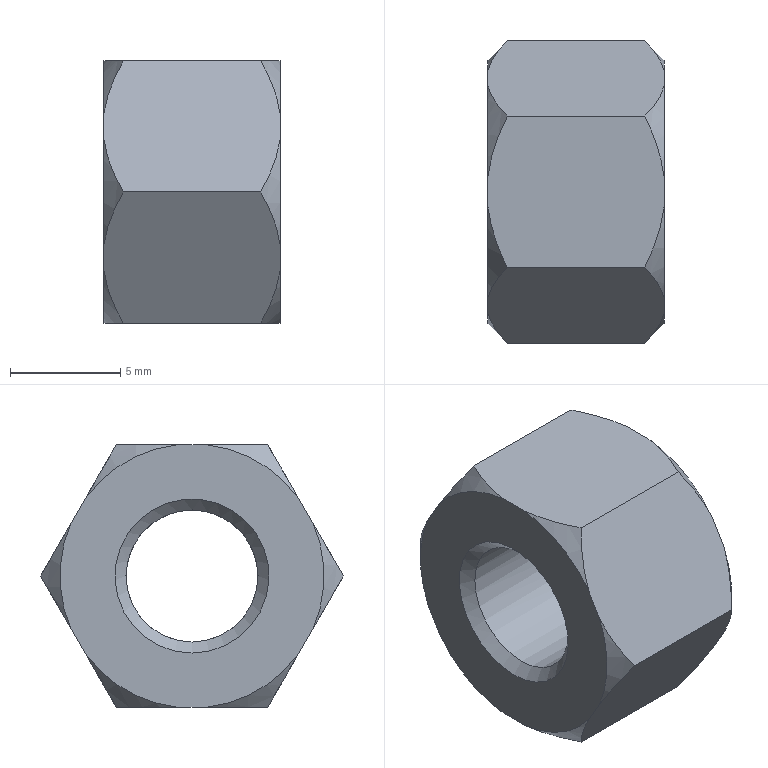Part | NX | features DATUM_CSYS 4, EXTRUDE 3, OFFSET_REGION 3, SKETCH 3, CHAMFER 2 | 1 solid | 23 faces | box 8 x 13.765 x 11.921 mm | volume 747.808 mm3 | cone 14 | plane 8 | cylinder 1 | commonest cylinder face diameters 6 x1
STEP:
#1=CARTESIAN_POINT('',(0.8823,3.441,5.96));
#2=VERTEX_POINT('',#1);
#3=CARTESIAN_POINT('',(0.,4.817,3.577));
#4=VERTEX_POINT('',#3);
#5=CARTESIAN_POINT('',(0.8823,3.441,5.96));
#6=CARTESIAN_POINT('',(0.4452,3.878,5.203));
#7=CARTESIAN_POINT('',(0.1117,4.331,4.419));
#8=CARTESIAN_POINT('',(0.,4.817,3.577));
#9=B_SPLINE_CURVE_WITH_KNOTS('',3,(#5,#6,#7,#8),.UNSPECIFIED.,.F.,.F.,(4,4),(0.,0.002889),.UNSPECIFIED.);
#10=EDGE_CURVE('',#2,#4,#9,.T.);
#11=ORIENTED_EDGE('',*,*,#10,.T.);
#12=CARTESIAN_POINT('',(0.,0.6895,5.96));
#13=VERTEX_POINT('',#12);
#14=CARTESIAN_POINT('',(0.,0.,0.));
#15=DIRECTION('',(1.,0.,0.));
#16=DIRECTION('',(0.,0.,-1.));
#17=AXIS2_PLACEMENT_3D('',#14,#15,#16);
#18=CIRCLE('',#17,6.);
#19=EDGE_CURVE('',#13,#4,#18,.F.);
#20=ORIENTED_EDGE('',*,*,#19,.F.);
#21=CARTESIAN_POINT('',(0.,0.6895,5.96));
#22=CARTESIAN_POINT('',(0.1096,1.643,5.96));
#23=CARTESIAN_POINT('',(0.4475,2.571,5.96));
#24=CARTESIAN_POINT('',(0.8823,3.441,5.96));
#25=B_SPLINE_CURVE_WITH_KNOTS('',3,(#21,#22,#23,#24),.UNSPECIFIED.,.F.,.F.,(4,4),(0.004251,0.007109),.UNSPECIFIED.);
#26=EDGE_CURVE('',#13,#2,#25,.T.);
#27=ORIENTED_EDGE('',*,*,#26,.T.);
#28=EDGE_LOOP('',(#11,#20,#27));
#29=FACE_BOUND('',#28,.T.);
#30=CARTESIAN_POINT('',(4.,0.,0.));
#31=DIRECTION('',(1.,0.,0.));
#32=DIRECTION('',(0.,0.,-1.));
#33=AXIS2_PLACEMENT_3D('',#30,#31,#32);
#34=CONICAL_SURFACE('',#33,10.,0.7854);
#35=ADVANCED_FACE('',(#29),#34,.T.);
#36=CARTESIAN_POINT('',(0.8823,-3.441,5.96));
#37=VERTEX_POINT('',#36);
#38=CARTESIAN_POINT('',(0.,-0.6895,5.96));
#39=VERTEX_POINT('',#38);
#40=CARTESIAN_POINT('',(0.8823,-3.441,5.96));
#41=CARTESIAN_POINT('',(0.4452,-2.567,5.96));
#42=CARTESIAN_POINT('',(0.1117,-1.662,5.96));
#43=CARTESIAN_POINT('',(0.,-0.6895,5.96));
#44=B_SPLINE_CURVE_WITH_KNOTS('',3,(#40,#41,#42,#43),.UNSPECIFIED.,.F.,.F.,(4,4),(0.,0.002889),.UNSPECIFIED.);
#45=EDGE_CURVE('',#37,#39,#44,.T.);
#46=ORIENTED_EDGE('',*,*,#45,.T.);
#47=CARTESIAN_POINT('',(0.,-4.817,3.577));
#48=VERTEX_POINT('',#47);
#49=CARTESIAN_POINT('',(0.,0.,0.));
#50=DIRECTION('',(1.,0.,0.));
#51=DIRECTION('',(0.,0.,-1.));
#52=AXIS2_PLACEMENT_3D('',#49,#50,#51);
#53=CIRCLE('',#52,6.);
#54=EDGE_CURVE('',#48,#39,#53,.F.);
#55=ORIENTED_EDGE('',*,*,#54,.F.);
#56=CARTESIAN_POINT('',(0.,-4.817,3.577));
#57=CARTESIAN_POINT('',(0.1096,-4.34,4.403));
#58=CARTESIAN_POINT('',(0.4475,-3.876,5.207));
#59=CARTESIAN_POINT('',(0.8823,-3.441,5.96));
#60=B_SPLINE_CURVE_WITH_KNOTS('',3,(#56,#57,#58,#59),.UNSPECIFIED.,.F.,.F.,(4,4),(0.004251,0.007109),.UNSPECIFIED.);
#61=EDGE_CURVE('',#48,#37,#60,.T.);
#62=ORIENTED_EDGE('',*,*,#61,.T.);
#63=EDGE_LOOP('',(#46,#55,#62));
#64=FACE_BOUND('',#63,.T.);
#65=CARTESIAN_POINT('',(4.,0.,0.));
#66=DIRECTION('',(1.,0.,0.));
#67=DIRECTION('',(0.,0.,-1.));
#68=AXIS2_PLACEMENT_3D('',#65,#66,#67);
#69=CONICAL_SURFACE('',#68,10.,0.7854);
#70=ADVANCED_FACE('',(#64),#69,.T.);
#71=CARTESIAN_POINT('',(0.8823,-6.882,0.));
#72=VERTEX_POINT('',#71);
#73=CARTESIAN_POINT('',(0.,-5.506,2.383));
#74=VERTEX_POINT('',#73);
#75=CARTESIAN_POINT('',(0.8823,-6.882,0.));
#76=CARTESIAN_POINT('',(0.4452,-6.445,0.757));
#77=CARTESIAN_POINT('',(0.1117,-5.993,1.541));
#78=CARTESIAN_POINT('',(0.,-5.506,2.383));
#79=B_SPLINE_CURVE_WITH_KNOTS('',3,(#75,#76,#77,#78),.UNSPECIFIED.,.F.,.F.,(4,4),(0.,0.002889),.UNSPECIFIED.);
#80=EDGE_CURVE('',#72,#74,#79,.T.);
#81=ORIENTED_EDGE('',*,*,#80,.T.);
#82=CARTESIAN_POINT('',(0.,-5.506,-2.383));
#83=VERTEX_POINT('',#82);
#84=CARTESIAN_POINT('',(0.,0.,0.));
#85=DIRECTION('',(1.,0.,0.));
#86=DIRECTION('',(0.,0.,-1.));
#87=AXIS2_PLACEMENT_3D('',#84,#85,#86);
#88=CIRCLE('',#87,6.);
#89=EDGE_CURVE('',#83,#74,#88,.F.);
#90=ORIENTED_EDGE('',*,*,#89,.F.);
#91=CARTESIAN_POINT('',(0.,-5.506,-2.383));
#92=CARTESIAN_POINT('',(0.1096,-5.983,-1.557));
#93=CARTESIAN_POINT('',(0.4475,-6.447,-0.7532));
#94=CARTESIAN_POINT('',(0.8823,-6.882,0.));
#95=B_SPLINE_CURVE_WITH_KNOTS('',3,(#91,#92,#93,#94),.UNSPECIFIED.,.F.,.F.,(4,4),(0.004251,0.007109),.UNSPECIFIED.);
#96=EDGE_CURVE('',#83,#72,#95,.T.);
#97=ORIENTED_EDGE('',*,*,#96,.T.);
#98=EDGE_LOOP('',(#81,#90,#97));
#99=FACE_BOUND('',#98,.T.);
#100=CARTESIAN_POINT('',(4.,0.,0.));
#101=DIRECTION('',(1.,0.,0.));
#102=DIRECTION('',(0.,0.,-1.));
#103=AXIS2_PLACEMENT_3D('',#100,#101,#102);
#104=CONICAL_SURFACE('',#103,10.,0.7854);
#105=ADVANCED_FACE('',(#99),#104,.T.);
#106=CARTESIAN_POINT('',(0.8823,-3.441,-5.96));
#107=VERTEX_POINT('',#106);
#108=CARTESIAN_POINT('',(0.,-4.817,-3.577));
#109=VERTEX_POINT('',#108);
#110=CARTESIAN_POINT('',(0.8823,-3.441,-5.96));
#111=CARTESIAN_POINT('',(0.4452,-3.878,-5.203));
#112=CARTESIAN_POINT('',(0.1117,-4.331,-4.419));
#113=CARTESIAN_POINT('',(0.,-4.817,-3.577));
#114=B_SPLINE_CURVE_WITH_KNOTS('',3,(#110,#111,#112,#113),.UNSPECIFIED.,.F.,.F.,(4,4),(0.,0.002889),.UNSPECIFIED.);
#115=EDGE_CURVE('',#107,#109,#114,.T.);
#116=ORIENTED_EDGE('',*,*,#115,.T.);
#117=CARTESIAN_POINT('',(0.,-0.6895,-5.96));
#118=VERTEX_POINT('',#117);
#119=CARTESIAN_POINT('',(0.,0.,0.));
#120=DIRECTION('',(1.,0.,0.));
#121=DIRECTION('',(0.,0.,-1.));
#122=AXIS2_PLACEMENT_3D('',#119,#120,#121);
#123=CIRCLE('',#122,6.);
#124=EDGE_CURVE('',#118,#109,#123,.F.);
#125=ORIENTED_EDGE('',*,*,#124,.F.);
#126=CARTESIAN_POINT('',(0.,-0.6895,-5.96));
#127=CARTESIAN_POINT('',(0.1096,-1.643,-5.96));
#128=CARTESIAN_POINT('',(0.4475,-2.571,-5.96));
#129=CARTESIAN_POINT('',(0.8823,-3.441,-5.96));
#130=B_SPLINE_CURVE_WITH_KNOTS('',3,(#126,#127,#128,#129),.UNSPECIFIED.,.F.,.F.,(4,4),(0.004251,0.007109),.UNSPECIFIED.);
#131=EDGE_CURVE('',#118,#107,#130,.T.);
#132=ORIENTED_EDGE('',*,*,#131,.T.);
#133=EDGE_LOOP('',(#116,#125,#132));
#134=FACE_BOUND('',#133,.T.);
#135=CARTESIAN_POINT('',(4.,0.,0.));
#136=DIRECTION('',(1.,0.,0.));
#137=DIRECTION('',(0.,0.,-1.));
#138=AXIS2_PLACEMENT_3D('',#135,#136,#137);
#139=CONICAL_SURFACE('',#138,10.,0.7854);
#140=ADVANCED_FACE('',(#134),#139,.T.);
#141=CARTESIAN_POINT('',(0.8823,3.441,-5.96));
#142=VERTEX_POINT('',#141);
#143=CARTESIAN_POINT('',(0.,0.6895,-5.96));
#144=VERTEX_POINT('',#143);
#145=CARTESIAN_POINT('',(0.8823,3.441,-5.96));
#146=CARTESIAN_POINT('',(0.4452,2.567,-5.96));
#147=CARTESIAN_POINT('',(0.1117,1.662,-5.96));
#148=CARTESIAN_POINT('',(0.,0.6895,-5.96));
#149=B_SPLINE_CURVE_WITH_KNOTS('',3,(#145,#146,#147,#148),.UNSPECIFIED.,.F.,.F.,(4,4),(0.,0.002889),.UNSPECIFIED.);
#150=EDGE_CURVE('',#142,#144,#149,.T.);
#151=ORIENTED_EDGE('',*,*,#150,.T.);
#152=CARTESIAN_POINT('',(0.,4.817,-3.577));
#153=VERTEX_POINT('',#152);
#154=CARTESIAN_POINT('',(0.,0.,0.));
#155=DIRECTION('',(1.,0.,0.));
#156=DIRECTION('',(0.,0.,-1.));
#157=AXIS2_PLACEMENT_3D('',#154,#155,#156);
#158=CIRCLE('',#157,6.);
#159=EDGE_CURVE('',#153,#144,#158,.F.);
#160=ORIENTED_EDGE('',*,*,#159,.F.);
#161=CARTESIAN_POINT('',(0.,4.817,-3.577));
#162=CARTESIAN_POINT('',(0.1096,4.34,-4.403));
#163=CARTESIAN_POINT('',(0.4475,3.876,-5.207));
#164=CARTESIAN_POINT('',(0.8823,3.441,-5.96));
#165=B_SPLINE_CURVE_WITH_KNOTS('',3,(#161,#162,#163,#164),.UNSPECIFIED.,.F.,.F.,(4,4),(0.004251,0.007109),.UNSPECIFIED.);
#166=EDGE_CURVE('',#153,#142,#165,.T.);
#167=ORIENTED_EDGE('',*,*,#166,.T.);
#168=EDGE_LOOP('',(#151,#160,#167));
#169=FACE_BOUND('',#168,.T.);
#170=CARTESIAN_POINT('',(4.,0.,0.));
#171=DIRECTION('',(1.,0.,0.));
#172=DIRECTION('',(0.,0.,-1.));
#173=AXIS2_PLACEMENT_3D('',#170,#171,#172);
#174=CONICAL_SURFACE('',#173,10.,0.7854);
#175=ADVANCED_FACE('',(#169),#174,.T.);
#176=CARTESIAN_POINT('',(8.,4.817,3.577));
#177=VERTEX_POINT('',#176);
#178=CARTESIAN_POINT('',(8.,0.6895,5.96));
#179=VERTEX_POINT('',#178);
#180=CARTESIAN_POINT('',(8.,0.,0.));
#181=DIRECTION('',(1.,0.,0.));
#182=DIRECTION('',(0.,0.,-1.));
#183=AXIS2_PLACEMENT_3D('',#180,#181,#182);
#184=CIRCLE('',#183,6.);
#185=EDGE_CURVE('',#177,#179,#184,.T.);
#186=ORIENTED_EDGE('',*,*,#185,.F.);
#187=CARTESIAN_POINT('',(7.118,3.441,5.96));
#188=VERTEX_POINT('',#187);
#189=CARTESIAN_POINT('',(8.,4.817,3.577));
#190=CARTESIAN_POINT('',(7.89,4.34,4.403));
#191=CARTESIAN_POINT('',(7.553,3.876,5.207));
#192=CARTESIAN_POINT('',(7.118,3.441,5.96));
#193=B_SPLINE_CURVE_WITH_KNOTS('',3,(#189,#190,#191,#192),.UNSPECIFIED.,.F.,.F.,(4,4),(0.004251,0.007109),.UNSPECIFIED.);
#194=EDGE_CURVE('',#177,#188,#193,.T.);
#195=ORIENTED_EDGE('',*,*,#194,.T.);
#196=CARTESIAN_POINT('',(7.118,3.441,5.96));
#197=CARTESIAN_POINT('',(7.555,2.567,5.96));
#198=CARTESIAN_POINT('',(7.888,1.662,5.96));
#199=CARTESIAN_POINT('',(8.,0.6895,5.96));
#200=B_SPLINE_CURVE_WITH_KNOTS('',3,(#196,#197,#198,#199),.UNSPECIFIED.,.F.,.F.,(4,4),(0.,0.002889),.UNSPECIFIED.);
#201=EDGE_CURVE('',#188,#179,#200,.T.);
#202=ORIENTED_EDGE('',*,*,#201,.T.);
#203=EDGE_LOOP('',(#186,#195,#202));
#204=FACE_BOUND('',#203,.T.);
#205=CARTESIAN_POINT('',(8.,0.,0.));
#206=DIRECTION('',(-1.,0.,0.));
#207=DIRECTION('',(0.,0.,1.));
#208=AXIS2_PLACEMENT_3D('',#205,#206,#207);
#209=CONICAL_SURFACE('',#208,6.,0.7854);
#210=ADVANCED_FACE('',(#204),#209,.T.);
#211=CARTESIAN_POINT('',(8.,5.506,-2.383));
#212=VERTEX_POINT('',#211);
#213=CARTESIAN_POINT('',(8.,5.506,2.383));
#214=VERTEX_POINT('',#213);
#215=CARTESIAN_POINT('',(8.,0.,0.));
#216=DIRECTION('',(1.,0.,0.));
#217=DIRECTION('',(0.,0.,-1.));
#218=AXIS2_PLACEMENT_3D('',#215,#216,#217);
#219=CIRCLE('',#218,6.);
#220=EDGE_CURVE('',#212,#214,#219,.T.);
#221=ORIENTED_EDGE('',*,*,#220,.F.);
#222=CARTESIAN_POINT('',(7.118,6.882,0.));
#223=VERTEX_POINT('',#222);
#224=CARTESIAN_POINT('',(8.,5.506,-2.383));
#225=CARTESIAN_POINT('',(7.89,5.983,-1.557));
#226=CARTESIAN_POINT('',(7.553,6.447,-0.7532));
#227=CARTESIAN_POINT('',(7.118,6.882,0.));
#228=B_SPLINE_CURVE_WITH_KNOTS('',3,(#224,#225,#226,#227),.UNSPECIFIED.,.F.,.F.,(4,4),(0.004251,0.007109),.UNSPECIFIED.);
#229=EDGE_CURVE('',#212,#223,#228,.T.);
#230=ORIENTED_EDGE('',*,*,#229,.T.);
#231=CARTESIAN_POINT('',(7.118,6.882,0.));
#232=CARTESIAN_POINT('',(7.555,6.445,0.757));
#233=CARTESIAN_POINT('',(7.888,5.993,1.541));
#234=CARTESIAN_POINT('',(8.,5.506,2.383));
#235=B_SPLINE_CURVE_WITH_KNOTS('',3,(#231,#232,#233,#234),.UNSPECIFIED.,.F.,.F.,(4,4),(0.,0.002889),.UNSPECIFIED.);
#236=EDGE_CURVE('',#223,#214,#235,.T.);
#237=ORIENTED_EDGE('',*,*,#236,.T.);
#238=EDGE_LOOP('',(#221,#230,#237));
#239=FACE_BOUND('',#238,.T.);
#240=CARTESIAN_POINT('',(8.,0.,0.));
#241=DIRECTION('',(-1.,0.,0.));
#242=DIRECTION('',(0.,0.,1.));
#243=AXIS2_PLACEMENT_3D('',#240,#241,#242);
#244=CONICAL_SURFACE('',#243,6.,0.7854);
#245=ADVANCED_FACE('',(#239),#244,.T.);
#246=CARTESIAN_POINT('',(8.,0.6895,-5.96));
#247=VERTEX_POINT('',#246);
#248=CARTESIAN_POINT('',(8.,4.817,-3.577));
#249=VERTEX_POINT('',#248);
#250=CARTESIAN_POINT('',(8.,0.,0.));
#251=DIRECTION('',(1.,0.,0.));
#252=DIRECTION('',(0.,0.,-1.));
#253=AXIS2_PLACEMENT_3D('',#250,#251,#252);
#254=CIRCLE('',#253,6.);
#255=EDGE_CURVE('',#247,#249,#254,.T.);
#256=ORIENTED_EDGE('',*,*,#255,.F.);
#257=CARTESIAN_POINT('',(7.118,3.441,-5.96));
#258=VERTEX_POINT('',#257);
#259=CARTESIAN_POINT('',(8.,0.6895,-5.96));
#260=CARTESIAN_POINT('',(7.89,1.643,-5.96));
#261=CARTESIAN_POINT('',(7.553,2.571,-5.96));
#262=CARTESIAN_POINT('',(7.118,3.441,-5.96));
#263=B_SPLINE_CURVE_WITH_KNOTS('',3,(#259,#260,#261,#262),.UNSPECIFIED.,.F.,.F.,(4,4),(0.004251,0.007109),.UNSPECIFIED.);
#264=EDGE_CURVE('',#247,#258,#263,.T.);
#265=ORIENTED_EDGE('',*,*,#264,.T.);
#266=CARTESIAN_POINT('',(7.118,3.441,-5.96));
#267=CARTESIAN_POINT('',(7.555,3.878,-5.203));
#268=CARTESIAN_POINT('',(7.888,4.331,-4.419));
#269=CARTESIAN_POINT('',(8.,4.817,-3.577));
#270=B_SPLINE_CURVE_WITH_KNOTS('',3,(#266,#267,#268,#269),.UNSPECIFIED.,.F.,.F.,(4,4),(0.,0.002889),.UNSPECIFIED.);
#271=EDGE_CURVE('',#258,#249,#270,.T.);
#272=ORIENTED_EDGE('',*,*,#271,.T.);
#273=EDGE_LOOP('',(#256,#265,#272));
#274=FACE_BOUND('',#273,.T.);
#275=CARTESIAN_POINT('',(8.,0.,0.));
#276=DIRECTION('',(-1.,0.,0.));
#277=DIRECTION('',(0.,0.,1.));
#278=AXIS2_PLACEMENT_3D('',#275,#276,#277);
#279=CONICAL_SURFACE('',#278,6.,0.7854);
#280=ADVANCED_FACE('',(#274),#279,.T.);
#281=CARTESIAN_POINT('',(8.,-4.817,-3.577));
#282=VERTEX_POINT('',#281);
#283=CARTESIAN_POINT('',(8.,-0.6895,-5.96));
#284=VERTEX_POINT('',#283);
#285=CARTESIAN_POINT('',(8.,0.,0.));
#286=DIRECTION('',(1.,0.,0.));
#287=DIRECTION('',(0.,0.,-1.));
#288=AXIS2_PLACEMENT_3D('',#285,#286,#287);
#289=CIRCLE('',#288,6.);
#290=EDGE_CURVE('',#282,#284,#289,.T.);
#291=ORIENTED_EDGE('',*,*,#290,.F.);
#292=CARTESIAN_POINT('',(7.118,-3.441,-5.96));
#293=VERTEX_POINT('',#292);
#294=CARTESIAN_POINT('',(8.,-4.817,-3.577));
#295=CARTESIAN_POINT('',(7.89,-4.34,-4.403));
#296=CARTESIAN_POINT('',(7.553,-3.876,-5.207));
#297=CARTESIAN_POINT('',(7.118,-3.441,-5.96));
#298=B_SPLINE_CURVE_WITH_KNOTS('',3,(#294,#295,#296,#297),.UNSPECIFIED.,.F.,.F.,(4,4),(0.004251,0.007109),.UNSPECIFIED.);
#299=EDGE_CURVE('',#282,#293,#298,.T.);
#300=ORIENTED_EDGE('',*,*,#299,.T.);
#301=CARTESIAN_POINT('',(7.118,-3.441,-5.96));
#302=CARTESIAN_POINT('',(7.555,-2.567,-5.96));
#303=CARTESIAN_POINT('',(7.888,-1.662,-5.96));
#304=CARTESIAN_POINT('',(8.,-0.6895,-5.96));
#305=B_SPLINE_CURVE_WITH_KNOTS('',3,(#301,#302,#303,#304),.UNSPECIFIED.,.F.,.F.,(4,4),(0.,0.002889),.UNSPECIFIED.);
#306=EDGE_CURVE('',#293,#284,#305,.T.);
#307=ORIENTED_EDGE('',*,*,#306,.T.);
#308=EDGE_LOOP('',(#291,#300,#307));
#309=FACE_BOUND('',#308,.T.);
#310=CARTESIAN_POINT('',(8.,0.,0.));
#311=DIRECTION('',(-1.,0.,0.));
#312=DIRECTION('',(0.,0.,1.));
#313=AXIS2_PLACEMENT_3D('',#310,#311,#312);
#314=CONICAL_SURFACE('',#313,6.,0.7854);
#315=ADVANCED_FACE('',(#309),#314,.T.);
#316=CARTESIAN_POINT('',(8.,-5.506,2.383));
#317=VERTEX_POINT('',#316);
#318=CARTESIAN_POINT('',(8.,-5.506,-2.383));
#319=VERTEX_POINT('',#318);
#320=CARTESIAN_POINT('',(8.,0.,0.));
#321=DIRECTION('',(1.,0.,0.));
#322=DIRECTION('',(0.,0.,-1.));
#323=AXIS2_PLACEMENT_3D('',#320,#321,#322);
#324=CIRCLE('',#323,6.);
#325=EDGE_CURVE('',#317,#319,#324,.T.);
#326=ORIENTED_EDGE('',*,*,#325,.F.);
#327=CARTESIAN_POINT('',(7.118,-6.882,0.));
#328=VERTEX_POINT('',#327);
#329=CARTESIAN_POINT('',(8.,-5.506,2.383));
#330=CARTESIAN_POINT('',(7.89,-5.983,1.557));
#331=CARTESIAN_POINT('',(7.553,-6.447,0.7532));
#332=CARTESIAN_POINT('',(7.118,-6.882,0.));
#333=B_SPLINE_CURVE_WITH_KNOTS('',3,(#329,#330,#331,#332),.UNSPECIFIED.,.F.,.F.,(4,4),(0.004251,0.007109),.UNSPECIFIED.);
#334=EDGE_CURVE('',#317,#328,#333,.T.);
#335=ORIENTED_EDGE('',*,*,#334,.T.);
#336=CARTESIAN_POINT('',(7.118,-6.882,0.));
#337=CARTESIAN_POINT('',(7.555,-6.445,-0.757));
#338=CARTESIAN_POINT('',(7.888,-5.993,-1.541));
#339=CARTESIAN_POINT('',(8.,-5.506,-2.383));
#340=B_SPLINE_CURVE_WITH_KNOTS('',3,(#336,#337,#338,#339),.UNSPECIFIED.,.F.,.F.,(4,4),(0.,0.002889),.UNSPECIFIED.);
#341=EDGE_CURVE('',#328,#319,#340,.T.);
#342=ORIENTED_EDGE('',*,*,#341,.T.);
#343=EDGE_LOOP('',(#326,#335,#342));
#344=FACE_BOUND('',#343,.T.);
#345=CARTESIAN_POINT('',(8.,0.,0.));
#346=DIRECTION('',(-1.,0.,0.));
#347=DIRECTION('',(0.,0.,1.));
#348=AXIS2_PLACEMENT_3D('',#345,#346,#347);
#349=CONICAL_SURFACE('',#348,6.,0.7854);
#350=ADVANCED_FACE('',(#344),#349,.T.);
#351=CARTESIAN_POINT('',(8.,-0.6895,5.96));
#352=VERTEX_POINT('',#351);
#353=CARTESIAN_POINT('',(8.,5.,5.96));
#354=DIRECTION('',(0.,1.,0.));
#355=VECTOR('',#354,1000.);
#356=LINE('',#353,#355);
#357=EDGE_CURVE('',#179,#352,#356,.F.);
#358=ORIENTED_EDGE('',*,*,#357,.T.);
#359=CARTESIAN_POINT('',(8.,-4.817,3.577));
#360=VERTEX_POINT('',#359);
#361=CARTESIAN_POINT('',(8.,0.,0.));
#362=DIRECTION('',(1.,0.,0.));
#363=DIRECTION('',(0.,0.,-1.));
#364=AXIS2_PLACEMENT_3D('',#361,#362,#363);
#365=CIRCLE('',#364,6.);
#366=EDGE_CURVE('',#352,#360,#365,.T.);
#367=ORIENTED_EDGE('',*,*,#366,.T.);
#368=CARTESIAN_POINT('',(8.,-2.662,7.31));
#369=DIRECTION('',(0.,0.5,0.866));
#370=VECTOR('',#369,1000.);
#371=LINE('',#368,#370);
#372=EDGE_CURVE('',#360,#317,#371,.F.);
#373=ORIENTED_EDGE('',*,*,#372,.T.);
#374=ORIENTED_EDGE('',*,*,#325,.T.);
#375=CARTESIAN_POINT('',(8.,-7.662,1.35));
#376=DIRECTION('',(0.,-0.5,0.866));
#377=VECTOR('',#376,1000.);
#378=LINE('',#375,#377);
#379=EDGE_CURVE('',#319,#282,#378,.F.);
#380=ORIENTED_EDGE('',*,*,#379,.T.);
#381=ORIENTED_EDGE('',*,*,#290,.T.);
#382=CARTESIAN_POINT('',(8.,-5.,-5.96));
#383=DIRECTION('',(0.,-1.,0.));
#384=VECTOR('',#383,1000.);
#385=LINE('',#382,#384);
#386=EDGE_CURVE('',#284,#247,#385,.F.);
#387=ORIENTED_EDGE('',*,*,#386,.T.);
#388=ORIENTED_EDGE('',*,*,#255,.T.);
#389=CARTESIAN_POINT('',(8.,2.662,-7.31));
#390=DIRECTION('',(0.,-0.5,-0.866));
#391=VECTOR('',#390,1000.);
#392=LINE('',#389,#391);
#393=EDGE_CURVE('',#249,#212,#392,.F.);
#394=ORIENTED_EDGE('',*,*,#393,.T.);
#395=ORIENTED_EDGE('',*,*,#220,.T.);
#396=CARTESIAN_POINT('',(8.,7.662,-1.35));
#397=DIRECTION('',(0.,0.5,-0.866));
#398=VECTOR('',#397,1000.);
#399=LINE('',#396,#398);
#400=EDGE_CURVE('',#214,#177,#399,.F.);
#401=ORIENTED_EDGE('',*,*,#400,.T.);
#402=ORIENTED_EDGE('',*,*,#185,.T.);
#403=EDGE_LOOP('',(#358,#367,#373,#374,#380,#381,#387,#388,#394,#395,#401,#402));
#404=FACE_BOUND('',#403,.T.);
#405=CARTESIAN_POINT('',(8.,0.,-3.5));
#406=VERTEX_POINT('',#405);
#407=CARTESIAN_POINT('',(8.,0.,0.));
#408=DIRECTION('',(1.,0.,0.));
#409=DIRECTION('',(0.,0.,-1.));
#410=AXIS2_PLACEMENT_3D('',#407,#408,#409);
#411=CIRCLE('',#410,3.5);
#412=EDGE_CURVE('',#406,#406,#411,.F.);
#413=ORIENTED_EDGE('',*,*,#412,.T.);
#414=EDGE_LOOP('',(#413));
#415=FACE_BOUND('',#414,.T.);
#416=CARTESIAN_POINT('',(8.,0.,0.));
#417=DIRECTION('',(1.,0.,0.));
#418=DIRECTION('',(0.,0.,-1.));
#419=AXIS2_PLACEMENT_3D('',#416,#417,#418);
#420=PLANE('',#419);
#421=ADVANCED_FACE('',(#404,#415),#420,.T.);
#422=CARTESIAN_POINT('',(7.118,-3.441,5.96));
#423=VERTEX_POINT('',#422);
#424=CARTESIAN_POINT('',(7.118,-3.441,5.96));
#425=CARTESIAN_POINT('',(7.555,-3.878,5.203));
#426=CARTESIAN_POINT('',(7.888,-4.331,4.419));
#427=CARTESIAN_POINT('',(8.,-4.817,3.577));
#428=B_SPLINE_CURVE_WITH_KNOTS('',3,(#424,#425,#426,#427),.UNSPECIFIED.,.F.,.F.,(4,4),(0.,0.002889),.UNSPECIFIED.);
#429=EDGE_CURVE('',#423,#360,#428,.T.);
#430=ORIENTED_EDGE('',*,*,#429,.T.);
#431=ORIENTED_EDGE('',*,*,#366,.F.);
#432=CARTESIAN_POINT('',(8.,-0.6895,5.96));
#433=CARTESIAN_POINT('',(7.89,-1.643,5.96));
#434=CARTESIAN_POINT('',(7.553,-2.571,5.96));
#435=CARTESIAN_POINT('',(7.118,-3.441,5.96));
#436=B_SPLINE_CURVE_WITH_KNOTS('',3,(#432,#433,#434,#435),.UNSPECIFIED.,.F.,.F.,(4,4),(0.004251,0.007109),.UNSPECIFIED.);
#437=EDGE_CURVE('',#352,#423,#436,.T.);
#438=ORIENTED_EDGE('',*,*,#437,.T.);
#439=EDGE_LOOP('',(#430,#431,#438));
#440=FACE_BOUND('',#439,.T.);
#441=CARTESIAN_POINT('',(8.,0.,0.));
#442=DIRECTION('',(-1.,0.,0.));
#443=DIRECTION('',(0.,0.,1.));
#444=AXIS2_PLACEMENT_3D('',#441,#442,#443);
#445=CONICAL_SURFACE('',#444,6.,0.7854);
#446=ADVANCED_FACE('',(#440),#445,.T.);
#447=ORIENTED_EDGE('',*,*,#334,.F.);
#448=ORIENTED_EDGE('',*,*,#372,.F.);
#449=ORIENTED_EDGE('',*,*,#429,.F.);
#450=CARTESIAN_POINT('',(0.,-3.441,5.96));
#451=DIRECTION('',(1.,0.,0.));
#452=VECTOR('',#451,1000.);
#453=LINE('',#450,#452);
#454=EDGE_CURVE('',#37,#423,#453,.T.);
#455=ORIENTED_EDGE('',*,*,#454,.F.);
#456=ORIENTED_EDGE('',*,*,#61,.F.);
#457=CARTESIAN_POINT('',(0.,-5.162,2.98));
#458=DIRECTION('',(0.,-0.5,-0.866));
#459=VECTOR('',#458,1000.);
#460=LINE('',#457,#459);
#461=EDGE_CURVE('',#48,#74,#460,.T.);
#462=ORIENTED_EDGE('',*,*,#461,.T.);
#463=ORIENTED_EDGE('',*,*,#80,.F.);
#464=CARTESIAN_POINT('',(0.,-6.882,0.));
#465=DIRECTION('',(1.,0.,0.));
#466=VECTOR('',#465,1000.);
#467=LINE('',#464,#466);
#468=EDGE_CURVE('',#72,#328,#467,.T.);
#469=ORIENTED_EDGE('',*,*,#468,.T.);
#470=EDGE_LOOP('',(#447,#448,#449,#455,#456,#462,#463,#469));
#471=FACE_BOUND('',#470,.T.);
#472=CARTESIAN_POINT('',(0.,-2.662,7.31));
#473=DIRECTION('',(0.,-0.866,0.5));
#474=DIRECTION('',(0.,-0.5,-0.866));
#475=AXIS2_PLACEMENT_3D('',#472,#473,#474);
#476=PLANE('',#475);
#477=ADVANCED_FACE('',(#471),#476,.T.);
#478=ORIENTED_EDGE('',*,*,#437,.F.);
#479=ORIENTED_EDGE('',*,*,#357,.F.);
#480=ORIENTED_EDGE('',*,*,#201,.F.);
#481=CARTESIAN_POINT('',(0.,3.441,5.96));
#482=DIRECTION('',(1.,0.,0.));
#483=VECTOR('',#482,1000.);
#484=LINE('',#481,#483);
#485=EDGE_CURVE('',#2,#188,#484,.T.);
#486=ORIENTED_EDGE('',*,*,#485,.F.);
#487=ORIENTED_EDGE('',*,*,#26,.F.);
#488=CARTESIAN_POINT('',(0.,0.,5.96));
#489=DIRECTION('',(0.,-1.,0.));
#490=VECTOR('',#489,1000.);
#491=LINE('',#488,#490);
#492=EDGE_CURVE('',#13,#39,#491,.T.);
#493=ORIENTED_EDGE('',*,*,#492,.T.);
#494=ORIENTED_EDGE('',*,*,#45,.F.);
#495=ORIENTED_EDGE('',*,*,#454,.T.);
#496=EDGE_LOOP('',(#478,#479,#480,#486,#487,#493,#494,#495));
#497=FACE_BOUND('',#496,.T.);
#498=CARTESIAN_POINT('',(0.,5.,5.96));
#499=DIRECTION('',(0.,0.,1.));
#500=DIRECTION('',(0.,-1.,0.));
#501=AXIS2_PLACEMENT_3D('',#498,#499,#500);
#502=PLANE('',#501);
#503=ADVANCED_FACE('',(#497),#502,.T.);
#504=ORIENTED_EDGE('',*,*,#194,.F.);
#505=ORIENTED_EDGE('',*,*,#400,.F.);
#506=ORIENTED_EDGE('',*,*,#236,.F.);
#507=CARTESIAN_POINT('',(0.8823,6.882,0.));
#508=VERTEX_POINT('',#507);
#509=CARTESIAN_POINT('',(0.,6.882,0.));
#510=DIRECTION('',(1.,0.,0.));
#511=VECTOR('',#510,1000.);
#512=LINE('',#509,#511);
#513=EDGE_CURVE('',#508,#223,#512,.T.);
#514=ORIENTED_EDGE('',*,*,#513,.F.);
#515=CARTESIAN_POINT('',(0.,5.506,2.383));
#516=VERTEX_POINT('',#515);
#517=CARTESIAN_POINT('',(0.,5.506,2.383));
#518=CARTESIAN_POINT('',(0.1096,5.983,1.557));
#519=CARTESIAN_POINT('',(0.4475,6.447,0.7532));
#520=CARTESIAN_POINT('',(0.8823,6.882,0.));
#521=B_SPLINE_CURVE_WITH_KNOTS('',3,(#517,#518,#519,#520),.UNSPECIFIED.,.F.,.F.,(4,4),(0.004251,0.007109),.UNSPECIFIED.);
#522=EDGE_CURVE('',#516,#508,#521,.T.);
#523=ORIENTED_EDGE('',*,*,#522,.F.);
#524=CARTESIAN_POINT('',(0.,5.162,2.98));
#525=DIRECTION('',(0.,-0.5,0.866));
#526=VECTOR('',#525,1000.);
#527=LINE('',#524,#526);
#528=EDGE_CURVE('',#516,#4,#527,.T.);
#529=ORIENTED_EDGE('',*,*,#528,.T.);
#530=ORIENTED_EDGE('',*,*,#10,.F.);
#531=ORIENTED_EDGE('',*,*,#485,.T.);
#532=EDGE_LOOP('',(#504,#505,#506,#514,#523,#529,#530,#531));
#533=FACE_BOUND('',#532,.T.);
#534=CARTESIAN_POINT('',(0.,7.662,-1.35));
#535=DIRECTION('',(0.,0.866,0.5));
#536=DIRECTION('',(0.,-0.5,0.866));
#537=AXIS2_PLACEMENT_3D('',#534,#535,#536);
#538=PLANE('',#537);
#539=ADVANCED_FACE('',(#533),#538,.T.);
#540=ORIENTED_EDGE('',*,*,#229,.F.);
#541=ORIENTED_EDGE('',*,*,#393,.F.);
#542=ORIENTED_EDGE('',*,*,#271,.F.);
#543=CARTESIAN_POINT('',(0.,3.441,-5.96));
#544=DIRECTION('',(1.,0.,0.));
#545=VECTOR('',#544,1000.);
#546=LINE('',#543,#545);
#547=EDGE_CURVE('',#142,#258,#546,.T.);
#548=ORIENTED_EDGE('',*,*,#547,.F.);
#549=ORIENTED_EDGE('',*,*,#166,.F.);
#550=CARTESIAN_POINT('',(0.,5.506,-2.383));
#551=VERTEX_POINT('',#550);
#552=CARTESIAN_POINT('',(0.,5.162,-2.98));
#553=DIRECTION('',(0.,0.5,0.866));
#554=VECTOR('',#553,1000.);
#555=LINE('',#552,#554);
#556=EDGE_CURVE('',#153,#551,#555,.T.);
#557=ORIENTED_EDGE('',*,*,#556,.T.);
#558=CARTESIAN_POINT('',(0.8823,6.882,0.));
#559=CARTESIAN_POINT('',(0.4452,6.445,-0.757));
#560=CARTESIAN_POINT('',(0.1117,5.993,-1.541));
#561=CARTESIAN_POINT('',(0.,5.506,-2.383));
#562=B_SPLINE_CURVE_WITH_KNOTS('',3,(#558,#559,#560,#561),.UNSPECIFIED.,.F.,.F.,(4,4),(0.,0.002889),.UNSPECIFIED.);
#563=EDGE_CURVE('',#508,#551,#562,.T.);
#564=ORIENTED_EDGE('',*,*,#563,.F.);
#565=ORIENTED_EDGE('',*,*,#513,.T.);
#566=EDGE_LOOP('',(#540,#541,#542,#548,#549,#557,#564,#565));
#567=FACE_BOUND('',#566,.T.);
#568=CARTESIAN_POINT('',(0.,2.662,-7.31));
#569=DIRECTION('',(0.,0.866,-0.5));
#570=DIRECTION('',(0.,0.5,0.866));
#571=AXIS2_PLACEMENT_3D('',#568,#569,#570);
#572=PLANE('',#571);
#573=ADVANCED_FACE('',(#567),#572,.T.);
#574=ORIENTED_EDGE('',*,*,#264,.F.);
#575=ORIENTED_EDGE('',*,*,#386,.F.);
#576=ORIENTED_EDGE('',*,*,#306,.F.);
#577=CARTESIAN_POINT('',(0.,-3.441,-5.96));
#578=DIRECTION('',(1.,0.,0.));
#579=VECTOR('',#578,1000.);
#580=LINE('',#577,#579);
#581=EDGE_CURVE('',#107,#293,#580,.T.);
#582=ORIENTED_EDGE('',*,*,#581,.F.);
#583=ORIENTED_EDGE('',*,*,#131,.F.);
#584=CARTESIAN_POINT('',(0.,0.,-5.96));
#585=DIRECTION('',(0.,1.,0.));
#586=VECTOR('',#585,1000.);
#587=LINE('',#584,#586);
#588=EDGE_CURVE('',#118,#144,#587,.T.);
#589=ORIENTED_EDGE('',*,*,#588,.T.);
#590=ORIENTED_EDGE('',*,*,#150,.F.);
#591=ORIENTED_EDGE('',*,*,#547,.T.);
#592=EDGE_LOOP('',(#574,#575,#576,#582,#583,#589,#590,#591));
#593=FACE_BOUND('',#592,.T.);
#594=CARTESIAN_POINT('',(0.,-5.,-5.96));
#595=DIRECTION('',(0.,0.,-1.));
#596=DIRECTION('',(0.,1.,0.));
#597=AXIS2_PLACEMENT_3D('',#594,#595,#596);
#598=PLANE('',#597);
#599=ADVANCED_FACE('',(#593),#598,.T.);
#600=ORIENTED_EDGE('',*,*,#299,.F.);
#601=ORIENTED_EDGE('',*,*,#379,.F.);
#602=ORIENTED_EDGE('',*,*,#341,.F.);
#603=ORIENTED_EDGE('',*,*,#468,.F.);
#604=ORIENTED_EDGE('',*,*,#96,.F.);
#605=CARTESIAN_POINT('',(0.,-5.162,-2.98));
#606=DIRECTION('',(0.,0.5,-0.866));
#607=VECTOR('',#606,1000.);
#608=LINE('',#605,#607);
#609=EDGE_CURVE('',#83,#109,#608,.T.);
#610=ORIENTED_EDGE('',*,*,#609,.T.);
#611=ORIENTED_EDGE('',*,*,#115,.F.);
#612=ORIENTED_EDGE('',*,*,#581,.T.);
#613=EDGE_LOOP('',(#600,#601,#602,#603,#604,#610,#611,#612));
#614=FACE_BOUND('',#613,.T.);
#615=CARTESIAN_POINT('',(0.,-7.662,1.35));
#616=DIRECTION('',(0.,-0.866,-0.5));
#617=DIRECTION('',(0.,0.5,-0.866));
#618=AXIS2_PLACEMENT_3D('',#615,#616,#617);
#619=PLANE('',#618);
#620=ADVANCED_FACE('',(#614),#619,.T.);
#621=ORIENTED_EDGE('',*,*,#556,.F.);
#622=ORIENTED_EDGE('',*,*,#159,.T.);
#623=ORIENTED_EDGE('',*,*,#588,.F.);
#624=ORIENTED_EDGE('',*,*,#124,.T.);
#625=ORIENTED_EDGE('',*,*,#609,.F.);
#626=ORIENTED_EDGE('',*,*,#89,.T.);
#627=ORIENTED_EDGE('',*,*,#461,.F.);
#628=ORIENTED_EDGE('',*,*,#54,.T.);
#629=ORIENTED_EDGE('',*,*,#492,.F.);
#630=ORIENTED_EDGE('',*,*,#19,.T.);
#631=ORIENTED_EDGE('',*,*,#528,.F.);
#632=CARTESIAN_POINT('',(0.,0.,0.));
#633=DIRECTION('',(1.,0.,0.));
#634=DIRECTION('',(0.,0.,-1.));
#635=AXIS2_PLACEMENT_3D('',#632,#633,#634);
#636=CIRCLE('',#635,6.);
#637=EDGE_CURVE('',#516,#551,#636,.F.);
#638=ORIENTED_EDGE('',*,*,#637,.T.);
#639=EDGE_LOOP('',(#621,#622,#623,#624,#625,#626,#627,#628,#629,#630,#631,#638));
#640=FACE_BOUND('',#639,.T.);
#641=CARTESIAN_POINT('',(0.,0.,-3.5));
#642=VERTEX_POINT('',#641);
#643=CARTESIAN_POINT('',(0.,0.,0.));
#644=DIRECTION('',(1.,0.,0.));
#645=DIRECTION('',(0.,0.,-1.));
#646=AXIS2_PLACEMENT_3D('',#643,#644,#645);
#647=CIRCLE('',#646,3.5);
#648=EDGE_CURVE('',#642,#642,#647,.T.);
#649=ORIENTED_EDGE('',*,*,#648,.T.);
#650=EDGE_LOOP('',(#649));
#651=FACE_BOUND('',#650,.T.);
#652=CARTESIAN_POINT('',(0.,0.,0.));
#653=DIRECTION('',(1.,0.,0.));
#654=DIRECTION('',(0.,0.,-1.));
#655=AXIS2_PLACEMENT_3D('',#652,#653,#654);
#656=PLANE('',#655);
#657=ADVANCED_FACE('',(#640,#651),#656,.F.);
#658=ORIENTED_EDGE('',*,*,#563,.T.);
#659=ORIENTED_EDGE('',*,*,#637,.F.);
#660=ORIENTED_EDGE('',*,*,#522,.T.);
#661=EDGE_LOOP('',(#658,#659,#660));
#662=FACE_BOUND('',#661,.T.);
#663=CARTESIAN_POINT('',(4.,0.,0.));
#664=DIRECTION('',(1.,0.,0.));
#665=DIRECTION('',(0.,0.,-1.));
#666=AXIS2_PLACEMENT_3D('',#663,#664,#665);
#667=CONICAL_SURFACE('',#666,10.,0.7854);
#668=ADVANCED_FACE('',(#662),#667,.T.);
#669=CARTESIAN_POINT('',(0.5,0.,3.));
#670=VERTEX_POINT('',#669);
#671=CARTESIAN_POINT('',(0.5,0.,0.));
#672=DIRECTION('',(-1.,0.,0.));
#673=DIRECTION('',(0.,0.,1.));
#674=AXIS2_PLACEMENT_3D('',#671,#672,#673);
#675=CIRCLE('',#674,3.);
#676=EDGE_CURVE('',#670,#670,#675,.T.);
#677=ORIENTED_EDGE('',*,*,#676,.T.);
#678=EDGE_LOOP('',(#677));
#679=FACE_BOUND('',#678,.T.);
#680=CARTESIAN_POINT('',(7.5,0.,-3.));
#681=VERTEX_POINT('',#680);
#682=CARTESIAN_POINT('',(7.5,0.,0.));
#683=DIRECTION('',(1.,0.,0.));
#684=DIRECTION('',(0.,0.,-1.));
#685=AXIS2_PLACEMENT_3D('',#682,#683,#684);
#686=CIRCLE('',#685,3.);
#687=EDGE_CURVE('',#681,#681,#686,.T.);
#688=ORIENTED_EDGE('',*,*,#687,.T.);
#689=EDGE_LOOP('',(#688));
#690=FACE_BOUND('',#689,.T.);
#691=CARTESIAN_POINT('',(-0.8,0.,0.));
#692=DIRECTION('',(1.,0.,0.));
#693=DIRECTION('',(0.,0.,-1.));
#694=AXIS2_PLACEMENT_3D('',#691,#692,#693);
#695=CYLINDRICAL_SURFACE('',#694,3.);
#696=ADVANCED_FACE('',(#679,#690),#695,.F.);
#697=ORIENTED_EDGE('',*,*,#648,.F.);
#698=EDGE_LOOP('',(#697));
#699=FACE_BOUND('',#698,.T.);
#700=ORIENTED_EDGE('',*,*,#676,.F.);
#701=EDGE_LOOP('',(#700));
#702=FACE_BOUND('',#701,.T.);
#703=CARTESIAN_POINT('',(0.5,0.,0.));
#704=DIRECTION('',(-1.,0.,0.));
#705=DIRECTION('',(0.,0.,1.));
#706=AXIS2_PLACEMENT_3D('',#703,#704,#705);
#707=CONICAL_SURFACE('',#706,3.,0.7854);
#708=ADVANCED_FACE('',(#699,#702),#707,.F.);
#709=ORIENTED_EDGE('',*,*,#412,.F.);
#710=EDGE_LOOP('',(#709));
#711=FACE_BOUND('',#710,.T.);
#712=ORIENTED_EDGE('',*,*,#687,.F.);
#713=EDGE_LOOP('',(#712));
#714=FACE_BOUND('',#713,.T.);
#715=CARTESIAN_POINT('',(7.5,0.,0.));
#716=DIRECTION('',(1.,0.,0.));
#717=DIRECTION('',(0.,0.,-1.));
#718=AXIS2_PLACEMENT_3D('',#715,#716,#717);
#719=CONICAL_SURFACE('',#718,3.,0.7854);
#720=ADVANCED_FACE('',(#711,#714),#719,.F.);
#721=CLOSED_SHELL('',(#35,#70,#105,#140,#175,#210,#245,#280,#315,#350,#421,#446,#477,#503,#539,#573,#599,#620,#657,#668,#696,#708,#720));
#722=MANIFOLD_SOLID_BREP('',#721);
#723=(LENGTH_UNIT()NAMED_UNIT(*)SI_UNIT(.MILLI.,.METRE.));
#724=UNCERTAINTY_MEASURE_WITH_UNIT(LENGTH_MEASURE(0.0508),#723,'','');
#725=(NAMED_UNIT(*)PLANE_ANGLE_UNIT()SI_UNIT($,.RADIAN.));
#726=(NAMED_UNIT(*)SI_UNIT($,.STERADIAN.)SOLID_ANGLE_UNIT());
#727=(GEOMETRIC_REPRESENTATION_CONTEXT(3)GLOBAL_UNCERTAINTY_ASSIGNED_CONTEXT((#724))GLOBAL_UNIT_ASSIGNED_CONTEXT((#723,#725,#726))REPRESENTATION_CONTEXT('',''));
#728=ADVANCED_BREP_SHAPE_REPRESENTATION('',(#722),#727);